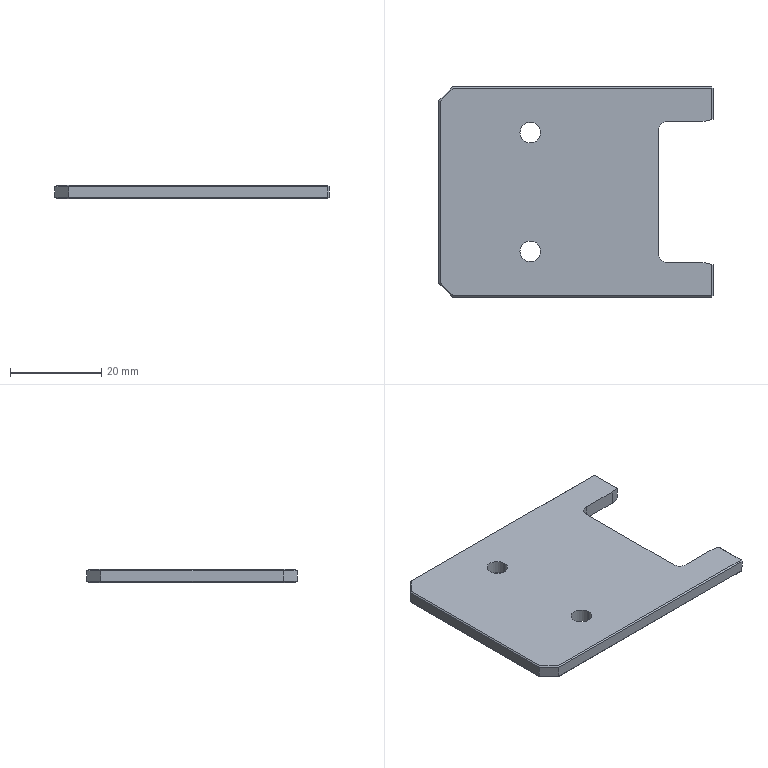Part | STEP file | A039 | 1 solid | 40 faces | box 60 x 46 x 3 mm | volume 7033 mm3 | plane 34 | cylinder 6 | commonest cylinder face diameters 4.5 x4 4 x2